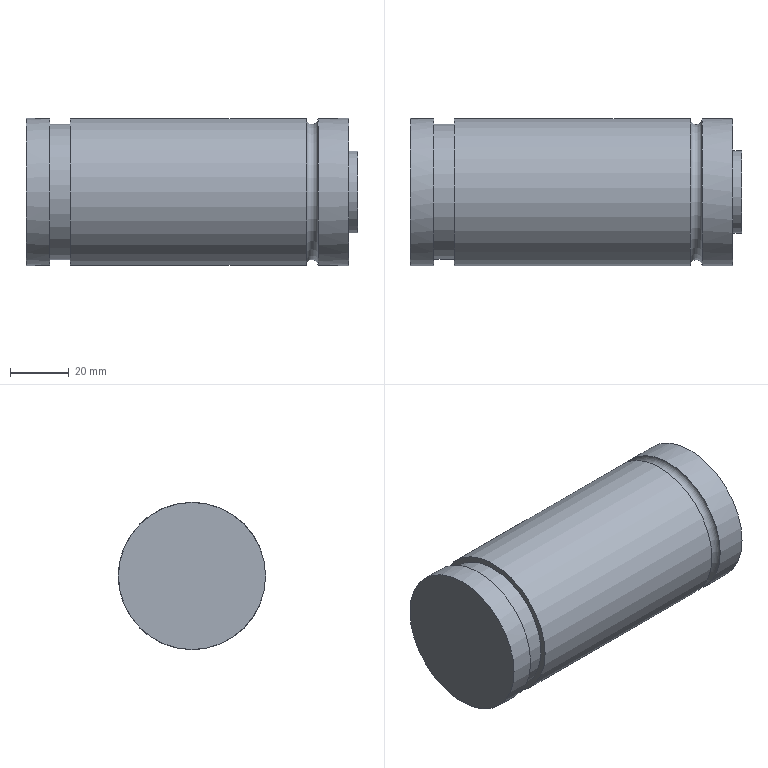Part | NX | features MAIN_BODY 2 | 1 solid | 11 faces | box 113 x 50.2 x 50.2 mm | volume 216486 mm3 | cylinder 5 | plane 5 | torus 1 | commonest cylinder face diameters 50.2 x3 28 x1 46.2 x1
STEP:
#1=CARTESIAN_POINT('',(797.,74.9,-330.));
#2=VERTEX_POINT('',#1);
#3=CARTESIAN_POINT('',(797.,100.,-330.));
#4=DIRECTION('',(-1.,0.,0.));
#5=DIRECTION('',(0.,-1.,0.));
#6=AXIS2_PLACEMENT_3D('',#3,#4,#5);
#7=CIRCLE('',#6,25.1);
#8=EDGE_CURVE('',#2,#2,#7,.F.);
#9=ORIENTED_EDGE('',*,*,#8,.T.);
#10=EDGE_LOOP('',(#9));
#11=FACE_BOUND('',#10,.T.);
#12=CARTESIAN_POINT('',(877.5,74.9,-330.));
#13=VERTEX_POINT('',#12);
#14=CARTESIAN_POINT('',(877.5,100.,-330.));
#15=DIRECTION('',(-1.,0.,0.));
#16=DIRECTION('',(0.,-1.,0.));
#17=AXIS2_PLACEMENT_3D('',#14,#15,#16);
#18=CIRCLE('',#17,25.1);
#19=EDGE_CURVE('',#13,#13,#18,.T.);
#20=ORIENTED_EDGE('',*,*,#19,.T.);
#21=EDGE_LOOP('',(#20));
#22=FACE_BOUND('',#21,.T.);
#23=CARTESIAN_POINT('',(892.,100.,-330.));
#24=DIRECTION('',(-1.,0.,0.));
#25=DIRECTION('',(0.,-1.,0.));
#26=AXIS2_PLACEMENT_3D('',#23,#24,#25);
#27=CYLINDRICAL_SURFACE('',#26,25.1);
#28=ADVANCED_FACE('',(#11,#22),#27,.T.);
#29=CARTESIAN_POINT('',(892.,125.1,-330.));
#30=VERTEX_POINT('',#29);
#31=CARTESIAN_POINT('',(892.,100.,-330.));
#32=DIRECTION('',(1.,0.,0.));
#33=DIRECTION('',(0.,1.,0.));
#34=AXIS2_PLACEMENT_3D('',#31,#32,#33);
#35=CIRCLE('',#34,25.1);
#36=EDGE_CURVE('',#30,#30,#35,.T.);
#37=ORIENTED_EDGE('',*,*,#36,.T.);
#38=EDGE_LOOP('',(#37));
#39=FACE_BOUND('',#38,.T.);
#40=CARTESIAN_POINT('',(892.,114.,-330.));
#41=VERTEX_POINT('',#40);
#42=CARTESIAN_POINT('',(892.,100.,-330.));
#43=DIRECTION('',(1.,0.,0.));
#44=DIRECTION('',(0.,1.,0.));
#45=AXIS2_PLACEMENT_3D('',#42,#43,#44);
#46=CIRCLE('',#45,14.);
#47=EDGE_CURVE('',#41,#41,#46,.T.);
#48=ORIENTED_EDGE('',*,*,#47,.F.);
#49=EDGE_LOOP('',(#48));
#50=FACE_BOUND('',#49,.T.);
#51=CARTESIAN_POINT('',(892.,100.,-330.));
#52=DIRECTION('',(1.,0.,0.));
#53=DIRECTION('',(0.,1.,0.));
#54=AXIS2_PLACEMENT_3D('',#51,#52,#53);
#55=PLANE('',#54);
#56=ADVANCED_FACE('',(#39,#50),#55,.T.);
#57=CARTESIAN_POINT('',(881.5,74.9,-330.));
#58=VERTEX_POINT('',#57);
#59=CARTESIAN_POINT('',(881.5,100.,-330.));
#60=DIRECTION('',(-1.,0.,0.));
#61=DIRECTION('',(0.,-1.,0.));
#62=AXIS2_PLACEMENT_3D('',#59,#60,#61);
#63=CIRCLE('',#62,25.1);
#64=EDGE_CURVE('',#58,#58,#63,.F.);
#65=ORIENTED_EDGE('',*,*,#64,.T.);
#66=EDGE_LOOP('',(#65));
#67=FACE_BOUND('',#66,.T.);
#68=ORIENTED_EDGE('',*,*,#36,.F.);
#69=EDGE_LOOP('',(#68));
#70=FACE_BOUND('',#69,.T.);
#71=CARTESIAN_POINT('',(892.,100.,-330.));
#72=DIRECTION('',(-1.,0.,0.));
#73=DIRECTION('',(0.,-1.,0.));
#74=AXIS2_PLACEMENT_3D('',#71,#72,#73);
#75=CYLINDRICAL_SURFACE('',#74,25.1);
#76=ADVANCED_FACE('',(#67,#70),#75,.T.);
#77=CARTESIAN_POINT('',(895.,114.,-330.));
#78=VERTEX_POINT('',#77);
#79=CARTESIAN_POINT('',(895.,100.,-330.));
#80=DIRECTION('',(1.,0.,0.));
#81=DIRECTION('',(0.,1.,0.));
#82=AXIS2_PLACEMENT_3D('',#79,#80,#81);
#83=CIRCLE('',#82,14.);
#84=EDGE_CURVE('',#78,#78,#83,.T.);
#85=ORIENTED_EDGE('',*,*,#84,.F.);
#86=EDGE_LOOP('',(#85));
#87=FACE_BOUND('',#86,.T.);
#88=ORIENTED_EDGE('',*,*,#47,.T.);
#89=EDGE_LOOP('',(#88));
#90=FACE_BOUND('',#89,.T.);
#91=CARTESIAN_POINT('',(895.,100.,-330.));
#92=DIRECTION('',(-1.,0.,0.));
#93=DIRECTION('',(0.,-1.,0.));
#94=AXIS2_PLACEMENT_3D('',#91,#92,#93);
#95=CYLINDRICAL_SURFACE('',#94,14.);
#96=ADVANCED_FACE('',(#87,#90),#95,.T.);
#97=ORIENTED_EDGE('',*,*,#84,.T.);
#98=EDGE_LOOP('',(#97));
#99=FACE_BOUND('',#98,.T.);
#100=CARTESIAN_POINT('',(895.,100.,-330.));
#101=DIRECTION('',(1.,0.,0.));
#102=DIRECTION('',(0.,1.,0.));
#103=AXIS2_PLACEMENT_3D('',#100,#101,#102);
#104=PLANE('',#103);
#105=ADVANCED_FACE('',(#99),#104,.T.);
#106=ORIENTED_EDGE('',*,*,#64,.F.);
#107=EDGE_LOOP('',(#106));
#108=FACE_BOUND('',#107,.T.);
#109=ORIENTED_EDGE('',*,*,#19,.F.);
#110=EDGE_LOOP('',(#109));
#111=FACE_BOUND('',#110,.T.);
#112=CARTESIAN_POINT('',(879.5,100.,-330.));
#113=DIRECTION('',(-1.,0.,0.));
#114=DIRECTION('',(0.,-1.,0.));
#115=AXIS2_PLACEMENT_3D('',#112,#113,#114);
#116=TOROIDAL_SURFACE('',#115,25.1,2.);
#117=ADVANCED_FACE('',(#108,#111),#116,.F.);
#118=CARTESIAN_POINT('',(797.,123.1,-330.));
#119=VERTEX_POINT('',#118);
#120=CARTESIAN_POINT('',(797.,100.,-330.));
#121=DIRECTION('',(1.,0.,0.));
#122=DIRECTION('',(0.,1.,0.));
#123=AXIS2_PLACEMENT_3D('',#120,#121,#122);
#124=CIRCLE('',#123,23.1);
#125=EDGE_CURVE('',#119,#119,#124,.T.);
#126=ORIENTED_EDGE('',*,*,#125,.T.);
#127=EDGE_LOOP('',(#126));
#128=FACE_BOUND('',#127,.T.);
#129=ORIENTED_EDGE('',*,*,#8,.F.);
#130=EDGE_LOOP('',(#129));
#131=FACE_BOUND('',#130,.T.);
#132=CARTESIAN_POINT('',(797.,100.,-330.));
#133=DIRECTION('',(-1.,0.,0.));
#134=DIRECTION('',(0.,-1.,0.));
#135=AXIS2_PLACEMENT_3D('',#132,#133,#134);
#136=PLANE('',#135);
#137=ADVANCED_FACE('',(#128,#131),#136,.T.);
#138=CARTESIAN_POINT('',(790.,123.1,-330.));
#139=VERTEX_POINT('',#138);
#140=CARTESIAN_POINT('',(790.,100.,-330.));
#141=DIRECTION('',(1.,0.,0.));
#142=DIRECTION('',(0.,1.,0.));
#143=AXIS2_PLACEMENT_3D('',#140,#141,#142);
#144=CIRCLE('',#143,23.1);
#145=EDGE_CURVE('',#139,#139,#144,.T.);
#146=ORIENTED_EDGE('',*,*,#145,.F.);
#147=EDGE_LOOP('',(#146));
#148=FACE_BOUND('',#147,.T.);
#149=CARTESIAN_POINT('',(790.,74.9,-330.));
#150=VERTEX_POINT('',#149);
#151=CARTESIAN_POINT('',(790.,100.,-330.));
#152=DIRECTION('',(-1.,0.,0.));
#153=DIRECTION('',(0.,-1.,0.));
#154=AXIS2_PLACEMENT_3D('',#151,#152,#153);
#155=CIRCLE('',#154,25.1);
#156=EDGE_CURVE('',#150,#150,#155,.T.);
#157=ORIENTED_EDGE('',*,*,#156,.F.);
#158=EDGE_LOOP('',(#157));
#159=FACE_BOUND('',#158,.T.);
#160=CARTESIAN_POINT('',(790.,100.,-330.));
#161=DIRECTION('',(-1.,0.,0.));
#162=DIRECTION('',(0.,-1.,0.));
#163=AXIS2_PLACEMENT_3D('',#160,#161,#162);
#164=PLANE('',#163);
#165=ADVANCED_FACE('',(#148,#159),#164,.F.);
#166=ORIENTED_EDGE('',*,*,#125,.F.);
#167=EDGE_LOOP('',(#166));
#168=FACE_BOUND('',#167,.T.);
#169=ORIENTED_EDGE('',*,*,#145,.T.);
#170=EDGE_LOOP('',(#169));
#171=FACE_BOUND('',#170,.T.);
#172=CARTESIAN_POINT('',(790.,100.,-330.));
#173=DIRECTION('',(1.,0.,0.));
#174=DIRECTION('',(0.,1.,0.));
#175=AXIS2_PLACEMENT_3D('',#172,#173,#174);
#176=CYLINDRICAL_SURFACE('',#175,23.1);
#177=ADVANCED_FACE('',(#168,#171),#176,.T.);
#178=CARTESIAN_POINT('',(782.,125.1,-330.));
#179=VERTEX_POINT('',#178);
#180=CARTESIAN_POINT('',(782.,100.,-330.));
#181=DIRECTION('',(1.,0.,0.));
#182=DIRECTION('',(0.,1.,0.));
#183=AXIS2_PLACEMENT_3D('',#180,#181,#182);
#184=CIRCLE('',#183,25.1);
#185=EDGE_CURVE('',#179,#179,#184,.T.);
#186=ORIENTED_EDGE('',*,*,#185,.F.);
#187=EDGE_LOOP('',(#186));
#188=FACE_BOUND('',#187,.T.);
#189=CARTESIAN_POINT('',(782.,100.,-330.));
#190=DIRECTION('',(1.,0.,0.));
#191=DIRECTION('',(0.,1.,0.));
#192=AXIS2_PLACEMENT_3D('',#189,#190,#191);
#193=PLANE('',#192);
#194=ADVANCED_FACE('',(#188),#193,.F.);
#195=ORIENTED_EDGE('',*,*,#156,.T.);
#196=EDGE_LOOP('',(#195));
#197=FACE_BOUND('',#196,.T.);
#198=ORIENTED_EDGE('',*,*,#185,.T.);
#199=EDGE_LOOP('',(#198));
#200=FACE_BOUND('',#199,.T.);
#201=CARTESIAN_POINT('',(892.,100.,-330.));
#202=DIRECTION('',(-1.,0.,0.));
#203=DIRECTION('',(0.,-1.,0.));
#204=AXIS2_PLACEMENT_3D('',#201,#202,#203);
#205=CYLINDRICAL_SURFACE('',#204,25.1);
#206=ADVANCED_FACE('',(#197,#200),#205,.T.);
#207=CLOSED_SHELL('',(#28,#56,#76,#96,#105,#117,#137,#165,#177,#194,#206));
#208=MANIFOLD_SOLID_BREP('',#207);
#209=(LENGTH_UNIT()NAMED_UNIT(*)SI_UNIT(.MILLI.,.METRE.));
#210=UNCERTAINTY_MEASURE_WITH_UNIT(LENGTH_MEASURE(0.00001),#209,'','');
#211=(NAMED_UNIT(*)PLANE_ANGLE_UNIT()SI_UNIT($,.RADIAN.));
#212=(NAMED_UNIT(*)SI_UNIT($,.STERADIAN.)SOLID_ANGLE_UNIT());
#213=(GEOMETRIC_REPRESENTATION_CONTEXT(3)GLOBAL_UNCERTAINTY_ASSIGNED_CONTEXT((#210))GLOBAL_UNIT_ASSIGNED_CONTEXT((#209,#211,#212))REPRESENTATION_CONTEXT('',''));
#214=ADVANCED_BREP_SHAPE_REPRESENTATION('',(#208),#213);